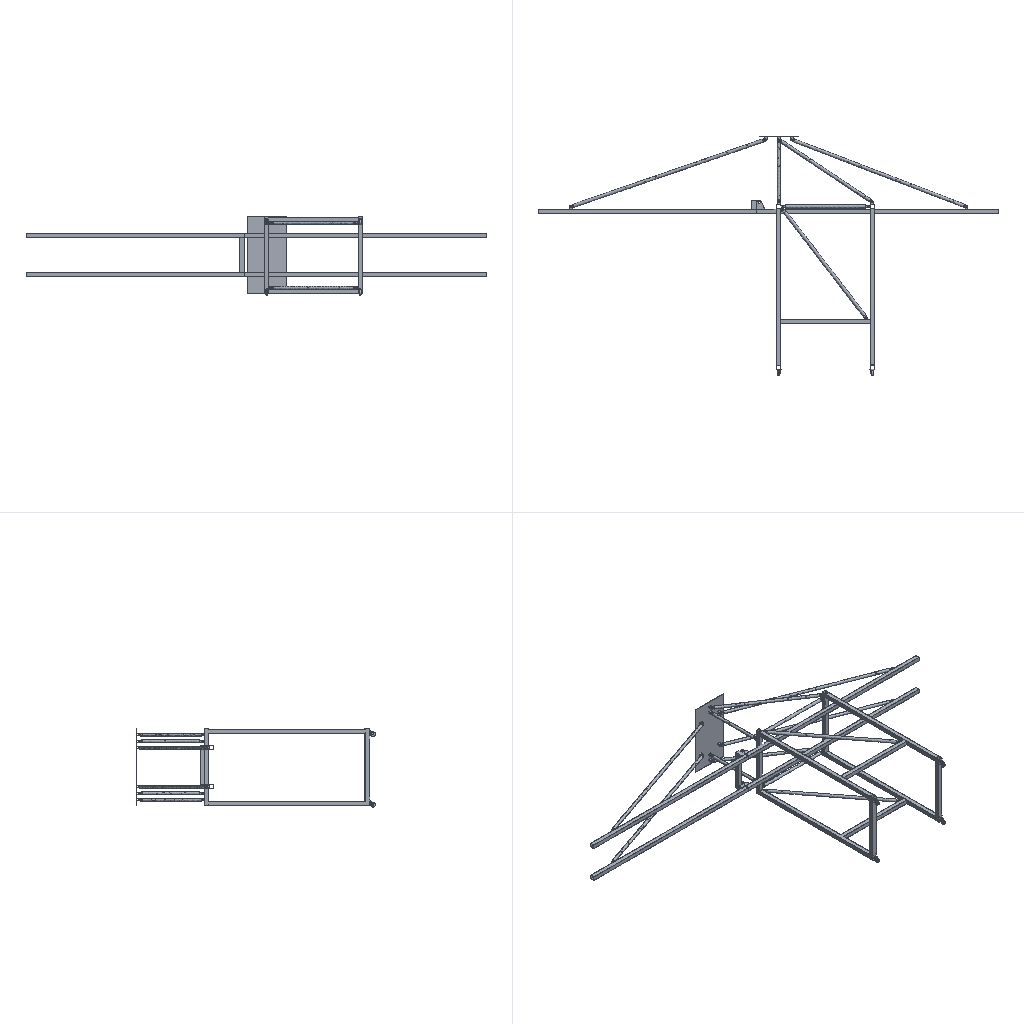Simulation study | ansys workbench
Ansys APDL input file, long lists of numbers shortened:
/batch
/config,noeldb,1     ! force off writing results to database
*get,_wallstrt,active,,time,wall
! ANSYS input file written by Workbench version 2021 R2
! File used for geometry attach:
/title,wbnew--____ 2 (C5)
! ****** Begin Custom Load Command Snippet ******
/COM, ACT Extensions:
/COM,     LSDYNA, 2021.1
/COM,
! ****** End   Custom Load Command Snippet ******
*DIM,_wb_ProjectScratch_dir,string,248
_wb_ProjectScratch_dir(1) = ''
*DIM,_wb_SolverFiles_dir,string,248
_wb_SolverFiles_dir(1) = ''
*DIM,_wb_userfiles_dir,string,248
_wb_userfiles_dir(1) = ''
/com,--- Data in consistent NMM units. See Solving Units in the help system for more information.
/units,MPA
/nopr
/wb,file,start              !  signify a WB generated input file
/prep7
! Turn off shape checking because checks already performed inside WB mesher.
! See help system for more information.
SHPP,OFF,,NOWARN
/nolist
etcon,set             ! allow ANSYS to choose best KEYOP's for 180x elements, resets any applicable keyopt to MAPDL defaults
/com,*********** Nodes for the whole assembly ***********
nblock,3,,390517
(1i9,3e20.9e3)
   266169    -5.195703030E+03    -1.862202026E+01    -3.149999976E+02
! (355015 more lines like these left out)
-1
/com,*********** Nodes for all Remote Points ***********
nblock,3
(1i9,3e20.9e3)
   355017    -5.215703010E+03     1.837798024E+01     2.999999970E+02
! (55 more lines like these left out)
-1
/wb,elem,start            !  set before creation of elements
/com,*********** Elements for Body 1 "0314-02__\Mirror2" ***********
et,1,187
eblock,19,solid,,2767
(19i9)
        1        1        1        1        0        0        0        0       10        0        1      724      768      864      772     4690     4916     4696     4691
! (5533 more lines like these left out)
-1
/com,*********** Elements for Body 2 "0314-02__\Mirror2" ***********
et,2,187
eblock,19,solid,,3150
(19i9)
        2        2        2        2        0        0        0        0       10        0     2768     6049     6117     6205     6154    10579    10946    10584    10581
! (6299 more lines like these left out)
-1
/com,*********** Elements for Body 3 "0314-02__\Mirror2" ***********
et,3,187
eblock,19,solid,,2799
(19i9)
        3        3        3        3        0        0        0        0       10        0     5918    11222    11224    11223    11993    12731    12735    12730    12734
! (5597 more lines like these left out)
-1
/com,*********** Elements for Body 4 "0314-02__\Mirror2" ***********
et,4,187
eblock,19,solid,,3118
(19i9)
        4        4        4        4        0        0        0        0       10        0     8717    17274    17316    17360    17346    22036    22204    22040    22038
! (6235 more lines like these left out)
-1
/com,*********** Elements for Body 5 "Component5\NONE" ***********
et,5,187
eblock,19,solid,,15574
(19i9)
        5        5        5        5        0        0        0        0       10        0    11835    22268    22271    27204    27193    27612    27640    27616    27614
! (31147 more lines like these left out)
-1
! (75 more sections like these left out)
/wb,elem,end               !  done creating elements
/com,*********** Send User Defined Coordinate System(s) ***********
local,12,0,-5215.703,18.378,300.,-180.,0.,-180.
local,13,0,-5215.703,18.378,-300.,-180.,0.,-180.
local,14,0,-2224.364,1048.374,300.,-180.,0.,-180.
local,15,0,-2224.364,1048.374,-300.,-180.,0.,-180.
local,16,0,-2024.364,1048.374,500.,0.,0.,0.
local,17,0,-2024.364,1048.374,400.,0.,0.,0.
local,18,0,-1824.364,1048.374,-300.,-180.,0.,-180.
local,19,0,-2024.364,1048.374,-500.,0.,0.,0.
local,20,0,-2024.364,1048.374,-400.,0.,0.,0.
local,21,0,-1824.364,1048.374,300.,0.,0.,0.
local,22,0,-2024.364,88.374,-400.,0.,0.,0.
local,23,0,-2024.364,88.374,400.,0.,0.,0.
local,24,0,-589.842,91.993,500.,0.,0.,0.
local,25,0,-589.842,91.993,-500.,0.,0.,0.
local,26,0,858.879,18.378,300.,0.,0.,0.
local,27,0,858.879,18.378,-300.,-180.,0.,-180.
local,28,0,-2324.363,83.378,-300.,-180.,0.,-180.
local,29,0,-2324.363,83.378,300.,0.,0.,0.
local,30,0,-1954.364,21.954,500.,-180.,0.,-180.
local,31,0,-1954.364,21.954,-500.,0.,0.,0.
local,32,0,-1954.364,-32.126,-552.5,0.,0.,0.
local,33,0,-1954.364,-32.126,552.5,0.,0.,0.
local,34,0,-659.864,21.954,500.,-180.,0.,-180.
local,35,0,-659.864,21.954,-500.,0.,0.,0.
local,36,0,-689.364,-1677.626,-552.5,-180.,0.,-180.
local,37,0,-689.364,-1677.626,552.5,-180.,0.,-180.
csys,0
toffst,273.15,  ! Temperature offset from absolute zero
/com,*********** Set Reference Temperature ***********
tref,22.
/wb,mat,start              !  starting to send materials
/com,*********** Send Materials ***********
Temperature = 'TEMP' ! Temperature
MP,DENS,1,7.85e-09,	! tonne mm^-3
MP,ALPX,1,1.2e-05,	! C^-1
MP,C,1,434000000,	! mm^2 s^-2 C^-1
MP,KXX,1,60.5,	! tonne mm s^-3 C^-1
MP,RSVX,1,0.00017,	! ohm mm
MP,EX,1,200000,	! tonne s^-2 mm^-1
MP,NUXY,1,0.3,
MP,MURX,1,10000,
Temperature = 'TEMP' ! Temperature
MP,DENS,2,7.85e-09,	! tonne mm^-3
MP,ALPX,2,1.2e-05,	! C^-1
MP,C,2,434000000,	! mm^2 s^-2 C^-1
MP,KXX,2,60.5,	! tonne mm s^-3 C^-1
MP,RSVX,2,0.00017,	! ohm mm
MP,EX,2,200000,	! tonne s^-2 mm^-1
MP,NUXY,2,0.3,
MP,MURX,2,10000,
Temperature = 'TEMP' ! Temperature
MP,DENS,3,7.85e-09,	! tonne mm^-3
MP,ALPX,3,1.2e-05,	! C^-1
MP,C,3,434000000,	! mm^2 s^-2 C^-1
MP,KXX,3,60.5,	! tonne mm s^-3 C^-1
MP,RSVX,3,0.00017,	! ohm mm
MP,EX,3,200000,	! tonne s^-2 mm^-1
MP,NUXY,3,0.3,
MP,MURX,3,10000,
Temperature = 'TEMP' ! Temperature
MP,DENS,4,7.85e-09,	! tonne mm^-3
MP,ALPX,4,1.2e-05,	! C^-1
MP,C,4,434000000,	! mm^2 s^-2 C^-1
MP,KXX,4,60.5,	! tonne mm s^-3 C^-1
MP,RSVX,4,0.00017,	! ohm mm
MP,EX,4,200000,	! tonne s^-2 mm^-1
MP,NUXY,4,0.3,
MP,MURX,4,10000,
Temperature = 'TEMP' ! Temperature
MP,DENS,5,7.85e-09,	! tonne mm^-3
MP,ALPX,5,1.2e-05,	! C^-1
MP,C,5,434000000,	! mm^2 s^-2 C^-1
MP,KXX,5,60.5,	! tonne mm s^-3 C^-1
MP,RSVX,5,0.00017,	! ohm mm
MP,EX,5,200000,	! tonne s^-2 mm^-1
MP,NUXY,5,0.3,
MP,MURX,5,10000,
Temperature = 'TEMP' ! Temperature
MP,DENS,6,7.85e-09,	! tonne mm^-3
MP,ALPX,6,1.2e-05,	! C^-1
MP,C,6,434000000,	! mm^2 s^-2 C^-1
MP,KXX,6,60.5,	! tonne mm s^-3 C^-1
MP,RSVX,6,0.00017,	! ohm mm
MP,EX,6,200000,	! tonne s^-2 mm^-1
MP,NUXY,6,0.3,
MP,MURX,6,10000,
Temperature = 'TEMP' ! Temperature
MP,DENS,7,7.85e-09,	! tonne mm^-3
MP,ALPX,7,1.2e-05,	! C^-1
MP,C,7,434000000,	! mm^2 s^-2 C^-1
MP,KXX,7,60.5,	! tonne mm s^-3 C^-1
MP,RSVX,7,0.00017,	! ohm mm
MP,EX,7,200000,	! tonne s^-2 mm^-1
MP,NUXY,7,0.3,
MP,MURX,7,10000,
Temperature = 'TEMP' ! Temperature
MP,DENS,8,7.85e-09,	! tonne mm^-3
MP,ALPX,8,1.2e-05,	! C^-1
MP,C,8,434000000,	! mm^2 s^-2 C^-1
MP,KXX,8,60.5,	! tonne mm s^-3 C^-1
MP,RSVX,8,0.00017,	! ohm mm
MP,EX,8,200000,	! tonne s^-2 mm^-1
MP,NUXY,8,0.3,
MP,MURX,8,10000,
Temperature = 'TEMP' ! Temperature
MP,DENS,9,7.85e-09,	! tonne mm^-3
MP,ALPX,9,1.2e-05,	! C^-1
MP,C,9,434000000,	! mm^2 s^-2 C^-1
MP,KXX,9,60.5,	! tonne mm s^-3 C^-1
MP,RSVX,9,0.00017,	! ohm mm
MP,EX,9,200000,	! tonne s^-2 mm^-1
! (641 more lines like these left out)
/wb,mat,end                !  done sending materials
/com,*********** Send Sheet Properties ***********
sectype,44,shell
secdata,4.
secoff,mid
sectype,45,shell
secdata,4.
secoff,mid
sectype,46,shell
secdata,4.
secoff,mid
sectype,47,shell
secdata,4.
secoff,mid
sectype,48,shell
secdata,4.
secoff,mid
sectype,49,shell
secdata,10.
secoff,mid
sectype,50,shell
secdata,10.
secoff,mid
sectype,51,shell
secdata,10.
secoff,mid
sectype,52,shell
secdata,10.
secoff,mid
sectype,53,shell
secdata,4.
secoff,mid
sectype,54,shell
secdata,4.
secoff,mid
sectype,55,shell
secdata,10.
secoff,mid
sectype,56,shell
secdata,10.
secoff,mid
sectype,57,shell
secdata,10.
secoff,mid
sectype,58,shell
secdata,10.
secoff,mid
sectype,59,shell
secdata,10.
secoff,mid
sectype,60,shell
secdata,10.
secoff,mid
sectype,61,shell
secdata,10.
secoff,mid
sectype,62,shell
secdata,10.
secoff,mid
sectype,63,shell
secdata,4.
secoff,mid
sectype,64,shell
secdata,4.
secoff,mid
sectype,65,shell
secdata,4.
secoff,mid
sectype,66,shell
secdata,4.
secoff,mid
sectype,67,shell
secdata,4.
secoff,mid
sectype,68,shell
secdata,4.
secoff,mid
sectype,69,shell
secdata,4.
secoff,mid
sectype,70,shell
! (96 more lines like these left out)
/wb,contact,start          !  starting to send contact
/com,*********** Create Contact "接触区域" ***********
/com,            Real Constant Set For Above Contact Is 82 & 81
*set,tid,82
*set,cid,81
r,tid
r,cid
et,tid,170
et,cid,174
eblock,10,,,515
(15i9)
   306125       82       82       82        0       10       15       16       16      961     1003       16      962
! (514 more lines like these left out)
-1
eblock,10,,,515
(15i9)
   306640       81       81       81        0       10       15       16       16      961     1003       16      962
! (514 more lines like these left out)
-1
eblock,10,,,119
(15i9)
   307155       81       82       81        0   337162   337163   337171   337170
! (118 more lines like these left out)
-1
eblock,10,,,119
(15i9)
   307274       82       81       82        0   337162   337163   337171   337170
! (118 more lines like these left out)
-1
keyo,cid,8,2               ! auto create asymmetric contact (from Program Controlled setting)
keyo,cid,10,0              ! adjust contact stiffness each NR iteration (from Program Controlled setting)
keyo,cid,12,5              ! bonded always
keyo,cid,18,1              ! small sliding turned on by application
keyo,cid,2,0               ! augmented Lagrange (from Program Controlled setting)
keyo,cid,4,0               ! on Gauss point (from Program Controlled setting)
keyo,cid,9,1               ! ignore initial gaps/penetration
keyo,cid,7,0               ! No Prediction
rmod,tid,3,10.      ! FKN
rmod,tid,5,0.       ! ICONT
rmod,tid,6,-20.121  ! PINB
rmod,tid,10,0.      ! CNOF
rmod,tid,12,0.      ! FKT
rmod,tid,36,721     ! WB DSID
rmod,cid,3,10.      ! FKN
rmod,cid,5,0.       ! ICONT
rmod,cid,6,-20.121  ! PINB
rmod,cid,10,0.      ! CNOF
rmod,cid,12,0.      ! FKT
rmod,cid,36,721     ! WB DSID
/com,*********** Create Contact "接触区域 2" ***********
/com,            Real Constant Set For Above Contact Is 84 & 83
*set,tid,84
*set,cid,83
r,tid
r,cid
et,tid,170
et,cid,174
eblock,10,,,511
(15i9)
   307393       84       84       84        0     5728     5249     5264     5264     6318     6314     5264     6426
! (510 more lines like these left out)
-1
eblock,10,,,511
(15i9)
   307904       83       83       83        0     5728     5249     5264     5264     6318     6314     5264     6426
! (510 more lines like these left out)
-1
eblock,10,,,98
(15i9)
   308415       83       84       83        0   332618   334222   334224   334223
! (97 more lines like these left out)
-1
eblock,10,,,98
(15i9)
   308513       84       83       84        0   332618   334222   334224   334223
! (97 more lines like these left out)
-1
keyo,cid,8,2               ! auto create asymmetric contact (from Program Controlled setting)
keyo,cid,10,0              ! adjust contact stiffness each NR iteration (from Program Controlled setting)
keyo,cid,12,5              ! bonded always
keyo,cid,18,1              ! small sliding turned on by application
keyo,cid,2,0               ! augmented Lagrange (from Program Controlled setting)
keyo,cid,4,0               ! on Gauss point (from Program Controlled setting)
keyo,cid,9,1               ! ignore initial gaps/penetration
keyo,cid,7,0               ! No Prediction
rmod,tid,3,10.      ! FKN
rmod,tid,5,0.       ! ICONT
rmod,tid,6,-20.121  ! PINB
rmod,tid,10,0.      ! CNOF
rmod,tid,12,0.      ! FKT
rmod,tid,36,724     ! WB DSID
rmod,cid,3,10.      ! FKN
rmod,cid,5,0.       ! ICONT
rmod,cid,6,-20.121  ! PINB
rmod,cid,10,0.      ! CNOF
rmod,cid,12,0.      ! FKT
rmod,cid,36,724     ! WB DSID
/com,*********** Create Contact "接触区域 3" ***********
/com,            Real Constant Set For Above Contact Is 86 & 85
*set,tid,86
*set,cid,85
r,tid
r,cid
et,tid,170
et,cid,174
eblock,10,,,509
(15i9)
   308611       86       86       86        0    11138    11617    11149    11149    12120    12195    11149    12113
! (508 more lines like these left out)
-1
eblock,10,,,509
(15i9)
   309120       85       85       85        0    11138    11617    11149    11149    12120    12195    11149    12113
! (508 more lines like these left out)
-1
eblock,10,,,119
(15i9)
   309629       85       86       85        0   321316   321317   321319   321318
! (118 more lines like these left out)
-1
eblock,10,,,119
(15i9)
   309748       86       85       86        0   321316   321317   321319   321318
! (118 more lines like these left out)
-1
keyo,cid,8,2               ! auto create asymmetric contact (from Program Controlled setting)
keyo,cid,10,0              ! adjust contact stiffness each NR iteration (from Program Controlled setting)
keyo,cid,12,5              ! bonded always
keyo,cid,18,1              ! small sliding turned on by application
keyo,cid,2,0               ! augmented Lagrange (from Program Controlled setting)
keyo,cid,4,0               ! on Gauss point (from Program Controlled setting)
keyo,cid,9,1               ! ignore initial gaps/penetration
keyo,cid,7,0               ! No Prediction
rmod,tid,3,10.      ! FKN
rmod,tid,5,0.       ! ICONT
rmod,tid,6,-20.121  ! PINB
rmod,tid,10,0.      ! CNOF
rmod,tid,12,0.      ! FKT
rmod,tid,36,727     ! WB DSID
rmod,cid,3,10.      ! FKN
rmod,cid,5,0.       ! ICONT
rmod,cid,6,-20.121  ! PINB
rmod,cid,10,0.      ! CNOF
rmod,cid,12,0.      ! FKT
rmod,cid,36,727     ! WB DSID
/com,*********** Create Contact "接触区域 4" ***********
/com,            Real Constant Set For Above Contact Is 88 & 87
*set,tid,88
*set,cid,87
r,tid
r,cid
et,tid,170
et,cid,174
eblock,10,,,511
(15i9)
   309867       88       88       88        0    16417    16896    16428    16428    17486    17561    16428    17480
! (510 more lines like these left out)
-1
eblock,10,,,511
(15i9)
   310378       87       87       87        0    16417    16896    16428    16428    17486    17561    16428    17480
! (510 more lines like these left out)
-1
eblock,10,,,98
(15i9)
   310889       87       88       87        0   321252   321253   321255   321254
! (97 more lines like these left out)
-1
eblock,10,,,98
(15i9)
   310987       88       87       88        0   321252   321253   321255   321254
! (97 more lines like these left out)
-1
keyo,cid,8,2               ! auto create asymmetric contact (from Program Controlled setting)
keyo,cid,10,0              ! adjust contact stiffness each NR iteration (from Program Controlled setting)
keyo,cid,12,5              ! bonded always
keyo,cid,18,1              ! small sliding turned on by application
keyo,cid,2,0               ! augmented Lagrange (from Program Controlled setting)
keyo,cid,4,0               ! on Gauss point (from Program Controlled setting)
keyo,cid,9,1               ! ignore initial gaps/penetration
keyo,cid,7,0               ! No Prediction
rmod,tid,3,10.      ! FKN
rmod,tid,5,0.       ! ICONT
rmod,tid,6,-20.121  ! PINB
rmod,tid,10,0.      ! CNOF
rmod,tid,12,0.      ! FKT
rmod,tid,36,730     ! WB DSID
rmod,cid,3,10.      ! FKN
rmod,cid,5,0.       ! ICONT
rmod,cid,6,-20.121  ! PINB
rmod,cid,10,0.      ! CNOF
rmod,cid,12,0.      ! FKT
rmod,cid,36,730     ! WB DSID
/com,*********** Create Contact "接触区域" ***********
/com,            Real Constant Set For Above Contact Is 90 & 89
*set,tid,90
*set,cid,89
r,tid
r,cid
et,tid,170
et,cid,174
eblock,10,,,12
(15i9)
   311085       90       90       90        0   255665   255666   255579   255585   255992   255819   255818   255831
! (11 more lines like these left out)
-1
eblock,10,,,12
(15i9)
   311097       89       89       89        0   255665   255666   255579   255585   255992   255819   255818   255831
! (11 more lines like these left out)
-1
eblock,10,,,69
(15i9)
   311109       89       90       89        0   353611   353609   353605   353606
! (68 more lines like these left out)
-1
eblock,10,,,69
(15i9)
   311178       90       89       90        0   353611   353609   353605   353606
! (68 more lines like these left out)
-1
keyo,cid,8,2               ! auto create asymmetric contact (from Program Controlled setting)
keyo,cid,10,0              ! adjust contact stiffness each NR iteration (from Program Controlled setting)
keyo,cid,12,5              ! bonded always
keyo,cid,18,1              ! small sliding turned on by application
keyo,cid,2,0               ! augmented Lagrange (from Program Controlled setting)
keyo,cid,4,0               ! on Gauss point (from Program Controlled setting)
keyo,cid,9,1               ! ignore initial gaps/penetration
keyo,cid,7,0               ! No Prediction
rmod,tid,3,10.      ! FKN
rmod,tid,5,0.       ! ICONT
rmod,tid,6,-20.121  ! PINB
rmod,tid,10,0.      ! CNOF
rmod,tid,12,0.      ! FKT
rmod,tid,36,735     ! WB DSID
rmod,cid,3,10.      ! FKN
rmod,cid,5,0.       ! ICONT
rmod,cid,6,-20.121  ! PINB
rmod,cid,10,0.      ! CNOF
rmod,cid,12,0.      ! FKT
rmod,cid,36,735     ! WB DSID
! (15 more sections like these left out)
/wb,contact,end            !  done creating contacts
/golist
/wb,load,start             !  starting to send loads
/com,*********** Create Remote Point "内部远程点" ***********
! -------- Remote Point Used by "回转 - Component6\NONE 至 多个" --------
*set,tid,122
*set,cid,121
et,cid,174
et,tid,170
keyo,tid,2,1               ! Don't fix the pilot node
keyo,tid,4,111111
keyo,cid,12,5              ! Bonded Contact
keyo,cid,4,2               ! Rigid CERIG style load
keyo,cid,2,2               ! MPC style contact
eblock,10,,,14
(15i9)
   314909      121      121      121        0    53421    53420    58349    58349    58828    58833    58349    58839
! (13 more lines like these left out)
-1
*set,_npilot,355017
_npilot456=_npilot
type,tid
mat ,cid
real,cid
tshape,pilo
en,314923,_npilot
tshape
csys,12
nrot,355017
csys,0
/com,*********** Create Remote Point "内部远程点 2" ***********
! -------- Remote Point Used by "回转 - Component6\NONE 至 多个" --------
*set,tid,124
*set,cid,123
et,cid,175
et,tid,170
keyo,tid,2,1               ! Don't fix the pilot node
keyo,tid,4,111111
keyo,cid,12,5              ! Bonded Contact
keyo,cid,4,0               ! Rigid CERIG style load
keyo,cid,2,2               ! MPC style contact
mat,123
real,123
type,123
en,314924,274073
en,314925,274078
en,314926,274079
en,314927,274085
en,314928,274086
en,314929,274088
en,314930,274099
en,314931,274101
en,314932,274103
en,314933,274104
en,314934,274107
en,314935,274108
en,314936,274111
en,314937,274115
en,314938,274117
en,314939,274123
*set,_npilot,355018
_npilot457=_npilot
type,tid
mat ,cid
real,cid
tshape,pilo
en,314940,_npilot
tshape
csys,12
nrot,355018
csys,0
/com,*********** Create Remote Point "内部远程点 3" ***********
! -------- Remote Point Used by "回转 - Component5\NONE 至 多个" --------
*set,tid,126
*set,cid,125
et,cid,174
et,tid,170
keyo,tid,2,1               ! Don't fix the pilot node
keyo,tid,4,111111
keyo,cid,12,5              ! Bonded Contact
keyo,cid,4,2               ! Rigid CERIG style load
keyo,cid,2,2               ! MPC style contact
eblock,10,,,14
(15i9)
   314941      125      125      125        0    22274    22273    27189    27189    27653    27658    27189    27664
! (13 more lines like these left out)
-1
*set,_npilot,355019
_npilot460=_npilot
type,tid
mat ,cid
real,cid
tshape,pilo
en,314955,_npilot
tshape
csys,13
nrot,355019
csys,0
/com,*********** Create Remote Point "内部远程点 4" ***********
! -------- Remote Point Used by "回转 - Component5\NONE 至 多个" --------
*set,tid,128
*set,cid,127
et,cid,175
et,tid,170
keyo,tid,2,1               ! Don't fix the pilot node
keyo,tid,4,111111
keyo,cid,12,5              ! Bonded Contact
keyo,cid,4,0               ! Rigid CERIG style load
keyo,cid,2,2               ! MPC style contact
mat,127
real,127
type,127
en,314956,280176
en,314957,280177
en,314958,280180
en,314959,280181
en,314960,280184
en,314961,280188
en,314962,280190
en,314963,280196
en,314964,282259
en,314965,282264
en,314966,282265
en,314967,282271
en,314968,282272
en,314969,282274
en,314970,282285
en,314971,282287
*set,_npilot,355020
_npilot461=_npilot
type,tid
mat ,cid
real,cid
tshape,pilo
en,314972,_npilot
tshape
csys,13
nrot,355020
csys,0
/com,*********** Create Remote Point "内部远程点 5" ***********
! -------- Remote Point Used by "回转 - Component6\NONE 至 多个" --------
*set,tid,130
*set,cid,129
et,cid,174
et,tid,170
keyo,tid,2,1               ! Don't fix the pilot node
keyo,tid,4,111111
keyo,cid,12,5              ! Bonded Contact
keyo,cid,4,2               ! Rigid CERIG style load
keyo,cid,2,2               ! MPC style contact
eblock,10,,,16
(15i9)
   314973      129      129      129        0    58354    53412    58355    58355    58770    58771    58355    84613
! (15 more lines like these left out)
-1
*set,_npilot,355021
_npilot464=_npilot
type,tid
mat ,cid
real,cid
tshape,pilo
en,314989,_npilot
tshape
csys,14
nrot,355021
csys,0
! (51 more sections like these left out)
/com,*********** Create Joint "回转 - Component6\NONE 至 多个" ***********
/com,            Real Constant Set For Above Joint Is 233
! Joint Element Type Declaration and Definition using MPC184
*set,_jid,233
et,_jid,184
keyo,_jid,1,6           ! Revolute Joint
keyo,_jid,4,1           ! Z Axis is revolute axis
sectype,_jid, joint, revo, _wbjoint
secjoint,,12,12
mat,_jid
real,_jid
type,_jid
secnum,_jid
en,306043,355017,355018      ! body to body joint
/com,*********** Create Joint "回转 - Component5\NONE 至 多个" ***********
/com,            Real Constant Set For Above Joint Is 234
! Joint Element Type Declaration and Definition using MPC184
*set,_jid,234
et,_jid,184
keyo,_jid,1,6           ! Revolute Joint
keyo,_jid,4,1           ! Z Axis is revolute axis
sectype,_jid, joint, revo, _wbjoint
secjoint,,13,13
mat,_jid
real,_jid
type,_jid
secnum,_jid
en,306044,355019,355020      ! body to body joint
/com,*********** Create Joint "回转 - Component6\NONE 至 多个" ***********
/com,            Real Constant Set For Above Joint Is 235
! Joint Element Type Declaration and Definition using MPC184
*set,_jid,235
et,_jid,184
keyo,_jid,1,6           ! Revolute Joint
keyo,_jid,4,1           ! Z Axis is revolute axis
sectype,_jid, joint, revo, _wbjoint
secjoint,,14,14
mat,_jid
real,_jid
type,_jid
secnum,_jid
en,306045,355021,355022      ! body to body joint
/com,*********** Create Joint "回转 - Component5\NONE 至 多个" ***********
/com,            Real Constant Set For Above Joint Is 236
! Joint Element Type Declaration and Definition using MPC184
*set,_jid,236
et,_jid,184
keyo,_jid,1,6           ! Revolute Joint
keyo,_jid,4,1           ! Z Axis is revolute axis
sectype,_jid, joint, revo, _wbjoint
secjoint,,15,15
mat,_jid
real,_jid
type,_jid
secnum,_jid
en,306046,355023,355024      ! body to body joint
/com,*********** Create Joint "回转 - Component16\NONE 至 多个" ***********
/com,            Real Constant Set For Above Joint Is 237
! Joint Element Type Declaration and Definition using MPC184
*set,_jid,237
et,_jid,184
keyo,_jid,1,6           ! Revolute Joint
keyo,_jid,4,1           ! Z Axis is revolute axis
sectype,_jid, joint, revo, _wbjoint
secjoint,,16,16
mat,_jid
real,_jid
type,_jid
secnum,_jid
en,306047,355025,355026      ! body to body joint
! (21 more sections like these left out)
/com,*********** Define Force Using Surface Effect Elements ***********
local,38,0,0.,0.,0.,0.,0.,0.
csys,0
et,259,154
eblock,10,,,9834
(15i9)
   316191      259      259      259       38   284490   284489   284507   284507
! (9833 more lines like these left out)
-1
esel,s,type,,259
keyop,259,2,1                ! Apply load in local coordinate system
keyop,259,7,1                ! Use original area so load is constant in large deformation
esel,all
/com,*********** Construct Remote Displacement ***********
/com,*********** Construct Remote Displacement ***********
/com,*********** Construct Remote Displacement ***********
/com,*********** Construct Remote Displacement ***********
/COM,*** Create a component for all remote displacements ***
CMBLOCK,REMOTEDISPALL,NODE,        4
(8i10)
    355069    355070    355071    355072
/gst,on,on
fini
*get,_numnode,node,0,count
*get,_numelem,elem,0,count
*get, _MAXELEMNUM, elem, 0, NUM, MAX
*get, _MAXNODENUM, node, 0, NUM, MAX
*get, _MAXELEMTYPE, etyp, 0, NUM, MAX
*get, _MAXREALCONST, real, 0, NUM, MAX
/go
/wb,load,end               !  done creating loads
/com,--- Number of total nodes = %_numnode%
/com,--- Number of contact elements = 19844
/com,--- Number of spring elements = 0
/com,--- Number of bearing elements = 0
/com,--- Number of solid elements = 229058
/com,--- Number of condensed parts = 0
/com,--- Number of total elements = %_numelem%
*get,_wallbsol,active,,time,wall
/com,****************************************************************************
/com,*************************    SOLUTION       ********************************
/com,****************************************************************************
/solu
antype,0                   ! static analysis
_thickRatio=0.4     ! Ratio of thick parts in the model
eqsl,sparse,,,,,1
cntr,print,1               ! print out contact info and also make no initial contact an error
dmpoption,emat,no             ! Don't combine emat file for DANSYS
dmpoption,esav,no             ! Don't combine esav file for DANSYS
nldiag,cont,iter           ! print out contact info each equilibrium iteration
rescontrol,,none                 ! Do not keep any restart files
/com,****************************************************
/com,******************* SOLVE FOR LS 1 OF 1 ****************
esel,s,type,,259
nsle
sfe,all,1,pres,1,0.
sfe,all,2,pres,1,-1.08504117672947e-002
sfe,all,3,pres,1,0.
nsel,all
esel,all
d,355069,ux,0.
d,355069,uy,0.
d,355069,uz,0.
d,355070,ux,0.
d,355070,uy,0.
d,355071,uy,0.
d,355071,uz,0.
d,355072,uy,0.
/nopr
/gopr
nsub,1,1,1
time,1.
outres,erase
outres,all,none
outres,nsol,all,
outres,rsol,all
outres,eangl,all
outres,etmp,all
outres,veng,all
outres,strs,all,
outres,epel,all,
outres,eppl,all,
outres,cont,all,
/nopr
esel,s,type,,233
esel,a,type,,234,258
cm,_elmisc,elem
esel,all
/gopr
outres,misc,all,_elmisc
! *********** WB SOLVE COMMAND ***********
! check interactive state
*get,ANSINTER_,active,,int
*if,ANSINTER_,ne,0,then
/eof
*endif
solve
/com *************** Write FE CONNECTORS *********
CEWRITE,file,ce,,INTE
/com,****************************************************
/com,*************** FINISHED SOLVE FOR LS 1 *************
*get,_wallasol,active,,time,wall
/nopr
*get,_numnode,node,0,count
*get,_numelem,elem,0,count
*get, _MAXELEMNUM, elem, 0, NUM, MAX
*get, _MAXNODENUM, node, 0, NUM, MAX,,,INTERNAL
*get, _MAXELEMTYPE, etyp, 0, NUM, MAX
*get, _MAXREALCONST, real, 0, NUM, MAX
/gopr
/post1
xmlo,ENCODING,ISO-8859-1
xmlo,parm
/xml,parm,xml
fini
/gopr
*get,_walldone,active,,time,wall
_preptime=(_wallbsol-_wallstrt)*3600
_solvtime=(_wallasol-_wallbsol)*3600
_posttime=(_walldone-_wallasol)*3600
_totaltim=(_walldone-_wallstrt)*3600
*get,_dlbratio,active,0,solu,dlbr
*get,_combtime,active,0,solu,comb
*get,_ssmode,active,0,solu,ssmm
*get,_ndofs,active,0,solu,ndof
/com,--- Total number of nodes = %_numnode%
/com,--- Total number of elements = %_numelem%
/com,--- Element load balance ratio = %_dlbratio%
/com,--- Time to combine distributed files = %_combtime%
/com,--- Sparse memory mode = %_ssmode%
/com,--- Number of DOF = %_ndofs%
/wb,file,end               ! done with WB generated input